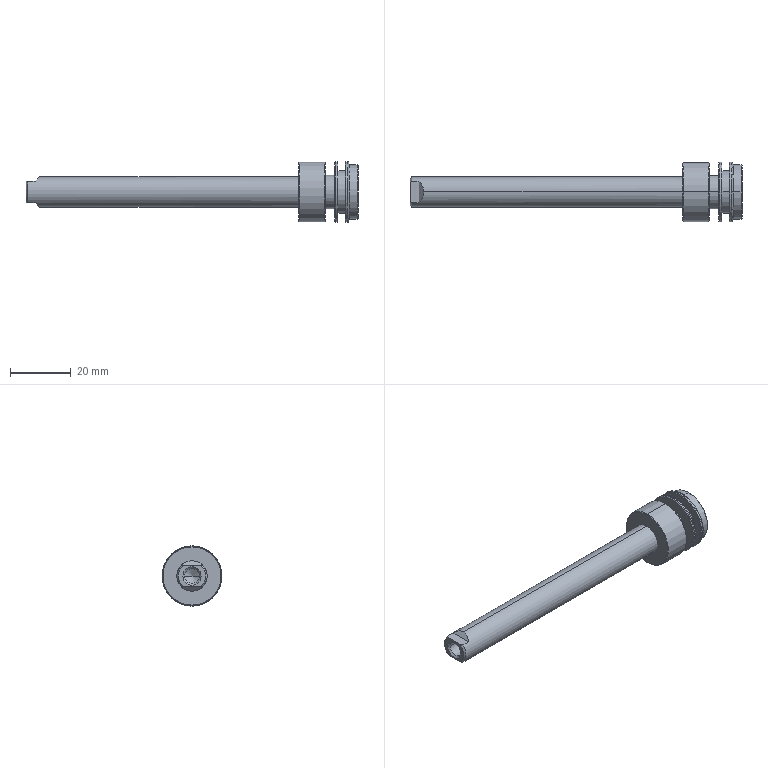Part | STEP file | TC_L_20x70_70r | 1 solid | 49 faces | box 109.5 x 19.9 x 19.9 mm | volume 11532 mm3 | cylinder 16 | cone 14 | plane 11 | torus 8 | commonest cylinder face diameters 19.9 x4 4.917 x2 10 x2 11 x2 14 x2 18 x2